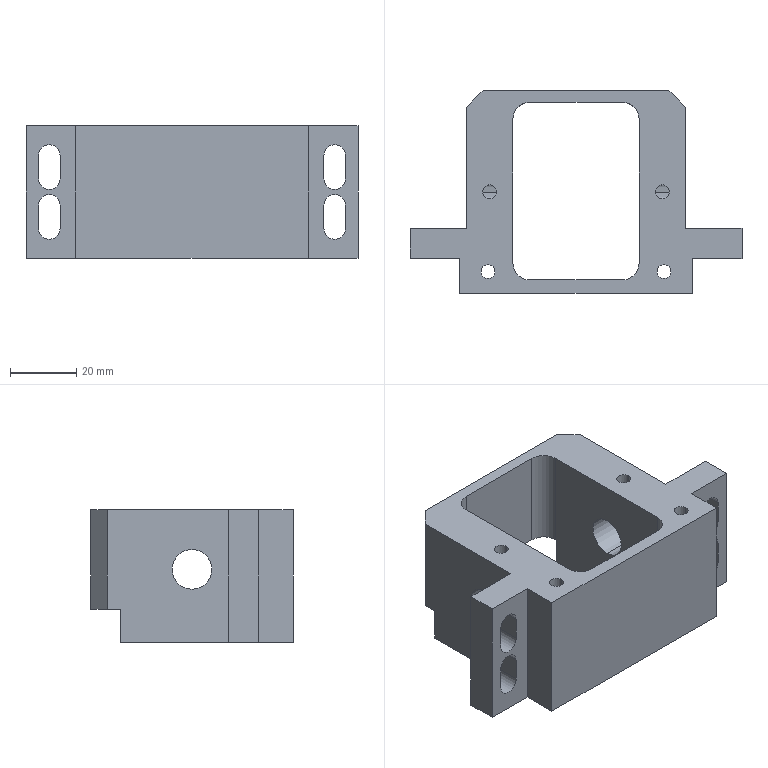Part | SolidWorks | features BaseBody 1 | 1 solid | 61 faces | box 100 x 61 x 40 mm | volume 80408 mm3 | plane 33 | cylinder 28 | commonest cylinder face diameters 4.2 x8 6.5 x8 10 x8 12 x4